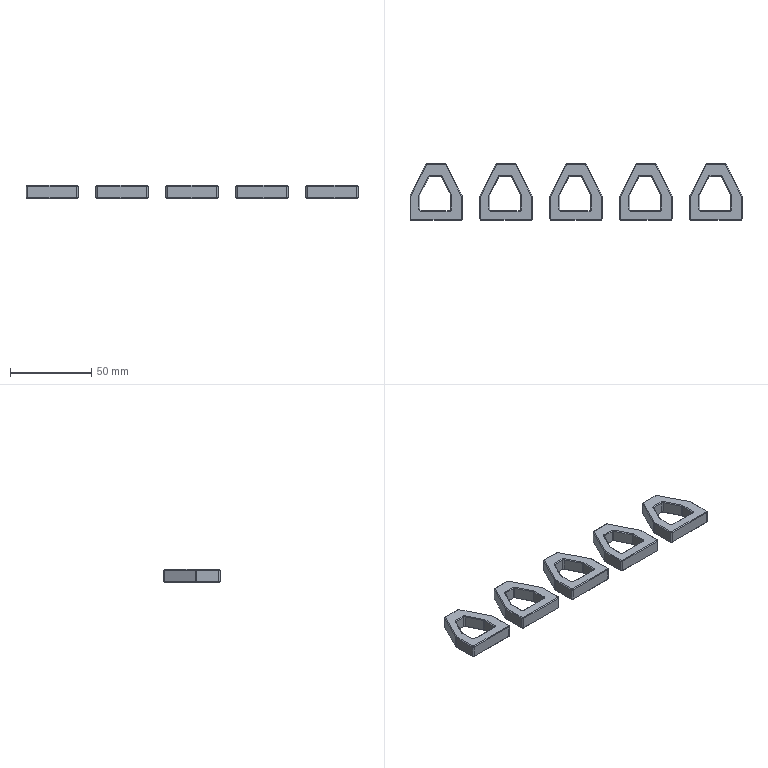Part | 5 solids | 470 faces | box 204 x 35 x 8 mm | volume 21796 mm3 | plane 210 | cone 160 | cylinder 100 | commonest cylinder face diameters 2 x60 4 x40